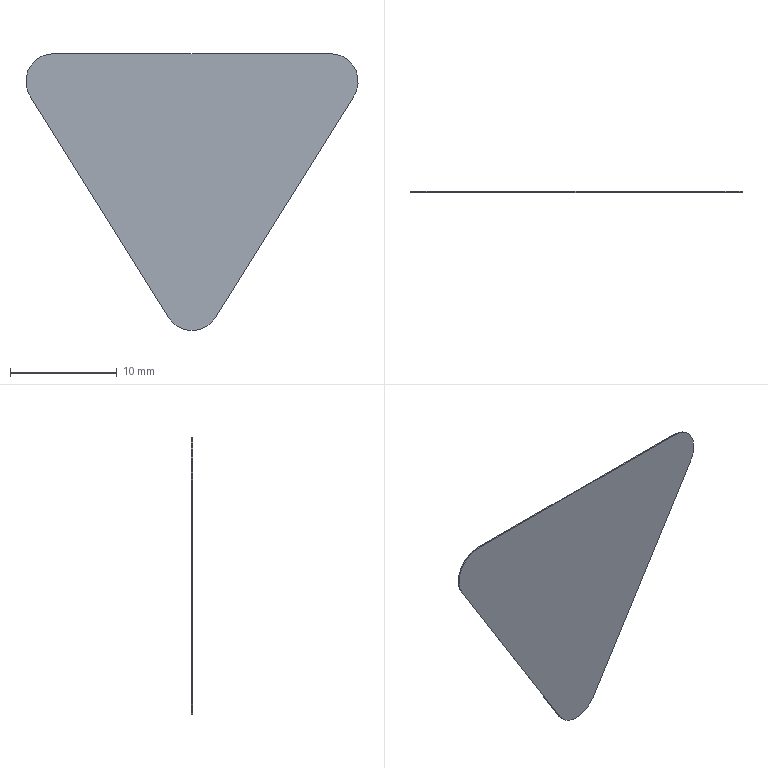Part | STEP file | basic_gh_motor_gh1_16 | 1 solid | 8 faces | box 31.17 x 0.11 x 25.975 mm | volume 53.443 mm3 | plane 5 | cylinder 3 | commonest cylinder face diameters 5.195 x3
STEP:
#1=CARTESIAN_POINT('',(-184.398,99.7,97.013));
#2=VERTEX_POINT('',#1);
#3=CARTESIAN_POINT('',(-186.6,99.7,93.038));
#4=VERTEX_POINT('',#3);
#5=CARTESIAN_POINT('',(-184.398,99.7,94.415));
#6=DIRECTION('',(0.,-1.,0.));
#7=DIRECTION('',(1.,0.,0.));
#8=AXIS2_PLACEMENT_3D('',#5,#6,#7);
#9=CIRCLE('',#8,2.598);
#10=EDGE_CURVE('',#2,#4,#9,.T.);
#11=ORIENTED_EDGE('',*,*,#10,.T.);
#12=CARTESIAN_POINT('',(-186.6,99.59,93.038));
#13=VERTEX_POINT('',#12);
#14=CARTESIAN_POINT('',(-186.6,99.59,93.038));
#15=DIRECTION('',(0.,1.,0.));
#16=VECTOR('',#15,1.);
#17=LINE('',#14,#16);
#18=EDGE_CURVE('',#13,#4,#17,.T.);
#19=ORIENTED_EDGE('',*,*,#18,.F.);
#20=CARTESIAN_POINT('',(-184.398,99.59,97.013));
#21=VERTEX_POINT('',#20);
#22=CARTESIAN_POINT('',(-184.398,99.59,94.415));
#23=DIRECTION('',(0.,1.,0.));
#24=DIRECTION('',(1.,0.,0.));
#25=AXIS2_PLACEMENT_3D('',#22,#23,#24);
#26=CIRCLE('',#25,2.598);
#27=EDGE_CURVE('',#13,#21,#26,.T.);
#28=ORIENTED_EDGE('',*,*,#27,.T.);
#29=CARTESIAN_POINT('',(-184.398,99.59,97.013));
#30=DIRECTION('',(0.,1.,0.));
#31=VECTOR('',#30,1.);
#32=LINE('',#29,#31);
#33=EDGE_CURVE('',#21,#2,#32,.T.);
#34=ORIENTED_EDGE('',*,*,#33,.T.);
#35=EDGE_LOOP('',(#11,#19,#28,#34));
#36=FACE_OUTER_BOUND('',#35,.T.);
#37=CARTESIAN_POINT('',(-184.398,99.59,94.415));
#38=DIRECTION('',(0.,1.,0.));
#39=DIRECTION('',(-0.8746,0.,0.4848));
#40=AXIS2_PLACEMENT_3D('',#37,#38,#39);
#41=CYLINDRICAL_SURFACE('',#40,2.598);
#42=ADVANCED_FACE('',(#36),#41,.T.);
#43=CARTESIAN_POINT('',(-173.613,99.7,72.258));
#44=VERTEX_POINT('',#43);
#45=CARTESIAN_POINT('',(-186.6,99.7,93.038));
#46=DIRECTION('',(0.53,0.,-0.848));
#47=VECTOR('',#46,1.);
#48=LINE('',#45,#47);
#49=EDGE_CURVE('',#4,#44,#48,.T.);
#50=ORIENTED_EDGE('',*,*,#49,.T.);
#51=CARTESIAN_POINT('',(-173.613,99.59,72.258));
#52=VERTEX_POINT('',#51);
#53=CARTESIAN_POINT('',(-173.613,99.59,72.258));
#54=DIRECTION('',(0.,1.,0.));
#55=VECTOR('',#54,1.);
#56=LINE('',#53,#55);
#57=EDGE_CURVE('',#52,#44,#56,.T.);
#58=ORIENTED_EDGE('',*,*,#57,.F.);
#59=CARTESIAN_POINT('',(-186.6,99.59,93.038));
#60=DIRECTION('',(0.53,0.,-0.848));
#61=VECTOR('',#60,1.);
#62=LINE('',#59,#61);
#63=EDGE_CURVE('',#13,#52,#62,.T.);
#64=ORIENTED_EDGE('',*,*,#63,.F.);
#65=ORIENTED_EDGE('',*,*,#18,.T.);
#66=EDGE_LOOP('',(#50,#58,#64,#65));
#67=FACE_OUTER_BOUND('',#66,.T.);
#68=CARTESIAN_POINT('',(-180.106,99.59,82.648));
#69=DIRECTION('',(-0.848,0.,-0.53));
#70=DIRECTION('',(-0.53,0.,0.848));
#71=AXIS2_PLACEMENT_3D('',#68,#69,#70);
#72=PLANE('',#71);
#73=ADVANCED_FACE('',(#67),#72,.T.);
#74=CARTESIAN_POINT('',(-169.207,99.7,72.258));
#75=VERTEX_POINT('',#74);
#76=CARTESIAN_POINT('',(-171.41,99.7,73.635));
#77=DIRECTION('',(0.,-1.,0.));
#78=DIRECTION('',(1.,0.,0.));
#79=AXIS2_PLACEMENT_3D('',#76,#77,#78);
#80=CIRCLE('',#79,2.598);
#81=EDGE_CURVE('',#44,#75,#80,.T.);
#82=ORIENTED_EDGE('',*,*,#81,.T.);
#83=CARTESIAN_POINT('',(-169.207,99.59,72.258));
#84=VERTEX_POINT('',#83);
#85=CARTESIAN_POINT('',(-169.207,99.59,72.258));
#86=DIRECTION('',(0.,1.,0.));
#87=VECTOR('',#86,1.);
#88=LINE('',#85,#87);
#89=EDGE_CURVE('',#84,#75,#88,.T.);
#90=ORIENTED_EDGE('',*,*,#89,.F.);
#91=CARTESIAN_POINT('',(-171.41,99.59,73.635));
#92=DIRECTION('',(0.,1.,0.));
#93=DIRECTION('',(1.,0.,0.));
#94=AXIS2_PLACEMENT_3D('',#91,#92,#93);
#95=CIRCLE('',#94,2.598);
#96=EDGE_CURVE('',#84,#52,#95,.T.);
#97=ORIENTED_EDGE('',*,*,#96,.T.);
#98=ORIENTED_EDGE('',*,*,#57,.T.);
#99=EDGE_LOOP('',(#82,#90,#97,#98));
#100=FACE_OUTER_BOUND('',#99,.T.);
#101=CARTESIAN_POINT('',(-171.41,99.59,73.635));
#102=DIRECTION('',(0.,1.,0.));
#103=DIRECTION('',(1.,0.,0.));
#104=AXIS2_PLACEMENT_3D('',#101,#102,#103);
#105=CYLINDRICAL_SURFACE('',#104,2.598);
#106=ADVANCED_FACE('',(#100),#105,.T.);
#107=CARTESIAN_POINT('',(-156.22,99.7,93.038));
#108=VERTEX_POINT('',#107);
#109=CARTESIAN_POINT('',(-156.22,99.7,93.038));
#110=DIRECTION('',(0.53,0.,0.848));
#111=VECTOR('',#110,1.);
#112=LINE('',#109,#111);
#113=EDGE_CURVE('',#75,#108,#112,.T.);
#114=ORIENTED_EDGE('',*,*,#113,.T.);
#115=CARTESIAN_POINT('',(-156.22,99.59,93.038));
#116=VERTEX_POINT('',#115);
#117=CARTESIAN_POINT('',(-156.22,99.59,93.038));
#118=DIRECTION('',(0.,1.,0.));
#119=VECTOR('',#118,1.);
#120=LINE('',#117,#119);
#121=EDGE_CURVE('',#116,#108,#120,.T.);
#122=ORIENTED_EDGE('',*,*,#121,.F.);
#123=CARTESIAN_POINT('',(-156.22,99.59,93.038));
#124=DIRECTION('',(-0.53,0.,-0.848));
#125=VECTOR('',#124,1.);
#126=LINE('',#123,#125);
#127=EDGE_CURVE('',#116,#84,#126,.T.);
#128=ORIENTED_EDGE('',*,*,#127,.T.);
#129=ORIENTED_EDGE('',*,*,#89,.T.);
#130=EDGE_LOOP('',(#114,#122,#128,#129));
#131=FACE_OUTER_BOUND('',#130,.T.);
#132=CARTESIAN_POINT('',(-162.714,99.59,82.648));
#133=DIRECTION('',(0.848,0.,-0.53));
#134=DIRECTION('',(-0.53,0.,-0.848));
#135=AXIS2_PLACEMENT_3D('',#132,#133,#134);
#136=PLANE('',#135);
#137=ADVANCED_FACE('',(#131),#136,.T.);
#138=CARTESIAN_POINT('',(-158.423,99.7,97.013));
#139=VERTEX_POINT('',#138);
#140=CARTESIAN_POINT('',(-158.423,99.7,94.415));
#141=DIRECTION('',(0.,-1.,0.));
#142=DIRECTION('',(1.,0.,0.));
#143=AXIS2_PLACEMENT_3D('',#140,#141,#142);
#144=CIRCLE('',#143,2.598);
#145=EDGE_CURVE('',#108,#139,#144,.T.);
#146=ORIENTED_EDGE('',*,*,#145,.T.);
#147=CARTESIAN_POINT('',(-158.423,99.59,97.013));
#148=VERTEX_POINT('',#147);
#149=CARTESIAN_POINT('',(-158.423,99.59,97.013));
#150=DIRECTION('',(0.,1.,0.));
#151=VECTOR('',#150,1.);
#152=LINE('',#149,#151);
#153=EDGE_CURVE('',#148,#139,#152,.T.);
#154=ORIENTED_EDGE('',*,*,#153,.F.);
#155=CARTESIAN_POINT('',(-158.423,99.59,94.415));
#156=DIRECTION('',(0.,1.,0.));
#157=DIRECTION('',(1.,0.,0.));
#158=AXIS2_PLACEMENT_3D('',#155,#156,#157);
#159=CIRCLE('',#158,2.598);
#160=EDGE_CURVE('',#148,#116,#159,.T.);
#161=ORIENTED_EDGE('',*,*,#160,.T.);
#162=ORIENTED_EDGE('',*,*,#121,.T.);
#163=EDGE_LOOP('',(#146,#154,#161,#162));
#164=FACE_OUTER_BOUND('',#163,.T.);
#165=CARTESIAN_POINT('',(-158.423,99.59,94.415));
#166=DIRECTION('',(0.,1.,0.));
#167=DIRECTION('',(1.,0.,0.));
#168=AXIS2_PLACEMENT_3D('',#165,#166,#167);
#169=CYLINDRICAL_SURFACE('',#168,2.598);
#170=ADVANCED_FACE('',(#164),#169,.T.);
#171=CARTESIAN_POINT('',(-184.398,99.7,97.013));
#172=DIRECTION('',(-1.,0.,0.));
#173=VECTOR('',#172,1.);
#174=LINE('',#171,#173);
#175=EDGE_CURVE('',#139,#2,#174,.T.);
#176=ORIENTED_EDGE('',*,*,#175,.T.);
#177=ORIENTED_EDGE('',*,*,#33,.F.);
#178=CARTESIAN_POINT('',(-184.398,99.59,97.013));
#179=DIRECTION('',(1.,0.,0.));
#180=VECTOR('',#179,1.);
#181=LINE('',#178,#180);
#182=EDGE_CURVE('',#21,#148,#181,.T.);
#183=ORIENTED_EDGE('',*,*,#182,.T.);
#184=ORIENTED_EDGE('',*,*,#153,.T.);
#185=EDGE_LOOP('',(#176,#177,#183,#184));
#186=FACE_OUTER_BOUND('',#185,.T.);
#187=CARTESIAN_POINT('',(-171.41,99.59,97.013));
#188=DIRECTION('',(0.,0.,1.));
#189=DIRECTION('',(1.,0.,0.));
#190=AXIS2_PLACEMENT_3D('',#187,#188,#189);
#191=PLANE('',#190);
#192=ADVANCED_FACE('',(#186),#191,.T.);
#193=ORIENTED_EDGE('',*,*,#10,.F.);
#194=ORIENTED_EDGE('',*,*,#175,.F.);
#195=ORIENTED_EDGE('',*,*,#145,.F.);
#196=ORIENTED_EDGE('',*,*,#113,.F.);
#197=ORIENTED_EDGE('',*,*,#81,.F.);
#198=ORIENTED_EDGE('',*,*,#49,.F.);
#199=EDGE_LOOP('',(#193,#194,#195,#196,#197,#198));
#200=FACE_OUTER_BOUND('',#199,.T.);
#201=CARTESIAN_POINT('',(-171.41,99.7,87.641));
#202=DIRECTION('',(0.,1.,0.));
#203=DIRECTION('',(1.,0.,0.));
#204=AXIS2_PLACEMENT_3D('',#201,#202,#203);
#205=PLANE('',#204);
#206=ADVANCED_FACE('',(#200),#205,.T.);
#207=ORIENTED_EDGE('',*,*,#182,.F.);
#208=ORIENTED_EDGE('',*,*,#27,.F.);
#209=ORIENTED_EDGE('',*,*,#63,.T.);
#210=ORIENTED_EDGE('',*,*,#96,.F.);
#211=ORIENTED_EDGE('',*,*,#127,.F.);
#212=ORIENTED_EDGE('',*,*,#160,.F.);
#213=EDGE_LOOP('',(#207,#208,#209,#210,#211,#212));
#214=FACE_OUTER_BOUND('',#213,.T.);
#215=CARTESIAN_POINT('',(-171.41,99.59,87.641));
#216=DIRECTION('',(0.,1.,0.));
#217=DIRECTION('',(1.,0.,0.));
#218=AXIS2_PLACEMENT_3D('',#215,#216,#217);
#219=PLANE('',#218);
#220=ADVANCED_FACE('',(#214),#219,.F.);
#221=CLOSED_SHELL('',(#42,#73,#106,#137,#170,#192,#206,#220));
#222=MANIFOLD_SOLID_BREP('',#221);
#223=(LENGTH_UNIT()NAMED_UNIT(*)SI_UNIT(.MILLI.,.METRE.));
#224=UNCERTAINTY_MEASURE_WITH_UNIT(LENGTH_MEASURE(0.01),#223,'','');
#225=(NAMED_UNIT(*)PLANE_ANGLE_UNIT()SI_UNIT($,.RADIAN.));
#226=(NAMED_UNIT(*)SI_UNIT($,.STERADIAN.)SOLID_ANGLE_UNIT());
#227=(GEOMETRIC_REPRESENTATION_CONTEXT(3)GLOBAL_UNCERTAINTY_ASSIGNED_CONTEXT((#224))GLOBAL_UNIT_ASSIGNED_CONTEXT((#223,#225,#226))REPRESENTATION_CONTEXT('',''));
#228=ADVANCED_BREP_SHAPE_REPRESENTATION('',(#222),#227);